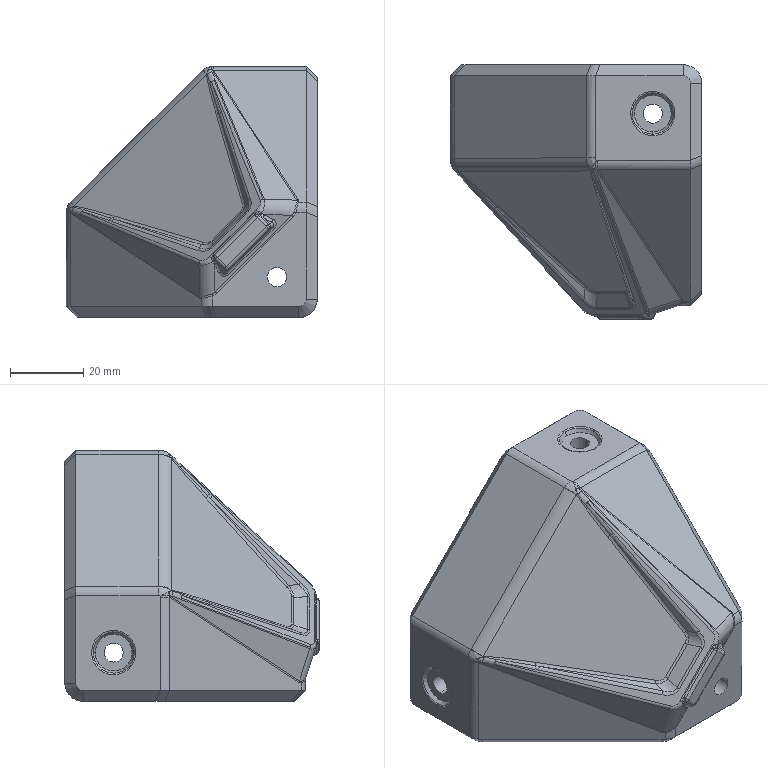Part | SolidWorks | features BaseBody 1 | 1 solid | 303 faces | box 68.413 x 69.253 x 68.359 mm | volume 36342 mm3 | cylinder 114 | plane 78 | spline 73 | sphere 19 | cone 11 | torus 8 | commonest cylinder face diameters 3 x33 8 x17 10 x14 5.2 x13 2 x10 1 x8